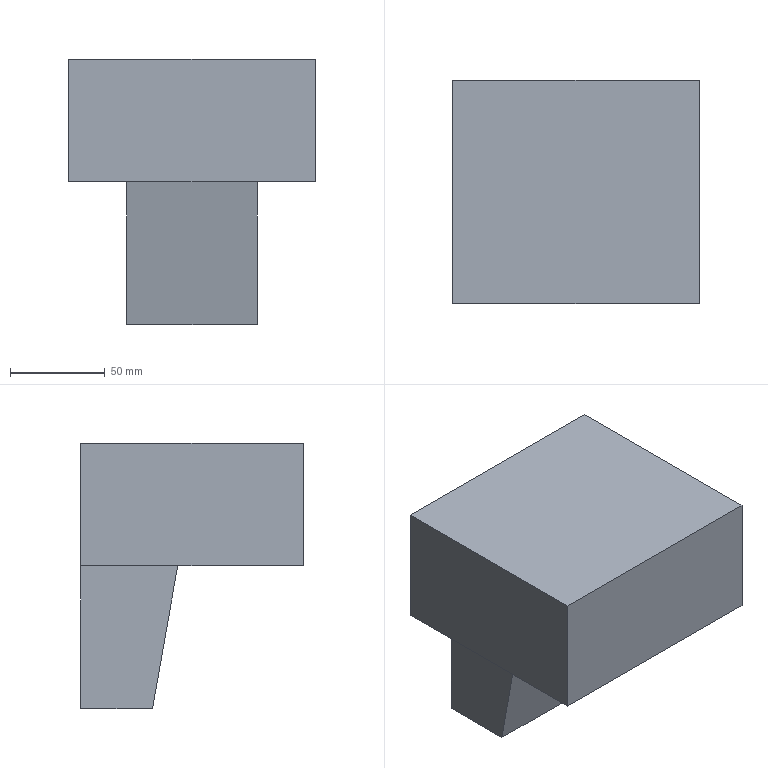Part | Creo | 1 solid | 10 faces | box 130 x 117.574 x 140 mm | volume 1218802 mm3 | plane 10
STEP:
#1=CARTESIAN_POINT('',(0.,0.,0.));
#2=DIRECTION('',(0.,0.,1.));
#3=DIRECTION('',(1.,0.,0.));
#4=AXIS2_PLACEMENT_3D('',#1,#2,#3);
#5=CARTESIAN_POINT('',(-59.275,152.799,-28.441));
#6=VERTEX_POINT('',#5);
#7=CARTESIAN_POINT('',(70.725,152.799,-28.441));
#8=VERTEX_POINT('',#7);
#9=CARTESIAN_POINT('',(-59.275,152.799,-28.441));
#10=DIRECTION('',(1.,0.000000015,0.));
#11=VECTOR('',#10,130.);
#12=LINE('',#9,#11);
#13=EDGE_CURVE('',#6,#8,#12,.T.);
#14=ORIENTED_EDGE('',*,*,#13,.T.);
#15=CARTESIAN_POINT('',(70.725,270.373,-28.441));
#16=VERTEX_POINT('',#15);
#17=CARTESIAN_POINT('',(70.725,270.373,-28.441));
#18=DIRECTION('',(0.,-1.,0.));
#19=VECTOR('',#18,117.574);
#20=LINE('',#17,#19);
#21=EDGE_CURVE('',#16,#8,#20,.T.);
#22=ORIENTED_EDGE('',*,*,#21,.F.);
#23=CARTESIAN_POINT('',(40.118,270.373,-28.441));
#24=VERTEX_POINT('',#23);
#25=CARTESIAN_POINT('',(70.725,270.373,-28.441));
#26=DIRECTION('',(-1.,0.,0.));
#27=VECTOR('',#26,30.607);
#28=LINE('',#25,#27);
#29=EDGE_CURVE('',#16,#24,#28,.T.);
#30=ORIENTED_EDGE('',*,*,#29,.T.);
#31=CARTESIAN_POINT('',(40.118,219.12,-28.441));
#32=VERTEX_POINT('',#31);
#33=CARTESIAN_POINT('',(40.118,219.12,-28.441));
#34=DIRECTION('',(0.,1.,0.));
#35=VECTOR('',#34,51.252);
#36=LINE('',#33,#35);
#37=EDGE_CURVE('',#32,#24,#36,.T.);
#38=ORIENTED_EDGE('',*,*,#37,.F.);
#39=CARTESIAN_POINT('',(-28.668,219.12,-28.441));
#40=VERTEX_POINT('',#39);
#41=CARTESIAN_POINT('',(-28.668,219.12,-28.441));
#42=DIRECTION('',(1.,0.,0.));
#43=VECTOR('',#42,68.786);
#44=LINE('',#41,#43);
#45=EDGE_CURVE('',#40,#32,#44,.T.);
#46=ORIENTED_EDGE('',*,*,#45,.F.);
#47=CARTESIAN_POINT('',(-28.668,270.373,-28.441));
#48=VERTEX_POINT('',#47);
#49=CARTESIAN_POINT('',(-28.668,270.373,-28.441));
#50=DIRECTION('',(0.,-1.,0.));
#51=VECTOR('',#50,51.252);
#52=LINE('',#49,#51);
#53=EDGE_CURVE('',#48,#40,#52,.T.);
#54=ORIENTED_EDGE('',*,*,#53,.F.);
#55=CARTESIAN_POINT('',(-59.275,270.373,-28.441));
#56=VERTEX_POINT('',#55);
#57=CARTESIAN_POINT('',(-28.668,270.373,-28.441));
#58=DIRECTION('',(-1.,0.,0.));
#59=VECTOR('',#58,30.607);
#60=LINE('',#57,#59);
#61=EDGE_CURVE('',#48,#56,#60,.T.);
#62=ORIENTED_EDGE('',*,*,#61,.T.);
#63=CARTESIAN_POINT('',(-59.275,270.373,-28.441));
#64=DIRECTION('',(0.,-1.,0.));
#65=VECTOR('',#64,117.574);
#66=LINE('',#63,#65);
#67=EDGE_CURVE('',#56,#6,#66,.T.);
#68=ORIENTED_EDGE('',*,*,#67,.T.);
#69=EDGE_LOOP('',(#14,#22,#30,#38,#46,#54,#62,#68));
#70=FACE_OUTER_BOUND('',#69,.F.);
#71=CARTESIAN_POINT('',(464.101,-434.627,-28.441));
#72=DIRECTION('',(0.,0.,-1.));
#73=DIRECTION('',(-1.,0.,0.));
#74=AXIS2_PLACEMENT_3D('',#71,#72,#73);
#75=PLANE('',#74);
#76=ADVANCED_FACE('',(#70),#75,.T.);
#77=CARTESIAN_POINT('',(-59.275,152.799,36.165));
#78=VERTEX_POINT('',#77);
#79=CARTESIAN_POINT('',(70.725,152.799,36.165));
#80=VERTEX_POINT('',#79);
#81=CARTESIAN_POINT('',(-59.275,152.799,36.165));
#82=DIRECTION('',(1.,0.000000015,0.));
#83=VECTOR('',#82,130.);
#84=LINE('',#81,#83);
#85=EDGE_CURVE('',#78,#80,#84,.T.);
#86=ORIENTED_EDGE('',*,*,#85,.T.);
#87=CARTESIAN_POINT('',(70.725,152.799,-28.441));
#88=DIRECTION('',(0.,0.,1.));
#89=VECTOR('',#88,64.606);
#90=LINE('',#87,#89);
#91=EDGE_CURVE('',#8,#80,#90,.T.);
#92=ORIENTED_EDGE('',*,*,#91,.F.);
#93=ORIENTED_EDGE('',*,*,#13,.F.);
#94=CARTESIAN_POINT('',(-59.275,152.799,-28.441));
#95=DIRECTION('',(0.,0.,1.));
#96=VECTOR('',#95,64.606);
#97=LINE('',#94,#96);
#98=EDGE_CURVE('',#6,#78,#97,.T.);
#99=ORIENTED_EDGE('',*,*,#98,.T.);
#100=EDGE_LOOP('',(#86,#92,#93,#99));
#101=FACE_OUTER_BOUND('',#100,.F.);
#102=CARTESIAN_POINT('',(57.885,152.799,12.059));
#103=DIRECTION('',(0.000000015,-1.,0.));
#104=DIRECTION('',(1.,0.000000015,0.));
#105=AXIS2_PLACEMENT_3D('',#102,#103,#104);
#106=PLANE('',#105);
#107=ADVANCED_FACE('',(#101),#106,.T.);
#108=CARTESIAN_POINT('',(-59.275,270.373,36.165));
#109=VERTEX_POINT('',#108);
#110=CARTESIAN_POINT('',(-59.275,270.373,36.165));
#111=DIRECTION('',(0.,-1.,0.));
#112=VECTOR('',#111,117.574);
#113=LINE('',#110,#112);
#114=EDGE_CURVE('',#109,#78,#113,.T.);
#115=ORIENTED_EDGE('',*,*,#114,.F.);
#116=CARTESIAN_POINT('',(70.725,270.373,36.165));
#117=VERTEX_POINT('',#116);
#118=CARTESIAN_POINT('',(70.725,270.373,36.165));
#119=DIRECTION('',(-1.,0.,0.));
#120=VECTOR('',#119,130.);
#121=LINE('',#118,#120);
#122=EDGE_CURVE('',#117,#109,#121,.T.);
#123=ORIENTED_EDGE('',*,*,#122,.F.);
#124=CARTESIAN_POINT('',(70.725,270.373,36.165));
#125=DIRECTION('',(0.,-1.,0.));
#126=VECTOR('',#125,117.574);
#127=LINE('',#124,#126);
#128=EDGE_CURVE('',#117,#80,#127,.T.);
#129=ORIENTED_EDGE('',*,*,#128,.T.);
#130=ORIENTED_EDGE('',*,*,#85,.F.);
#131=EDGE_LOOP('',(#115,#123,#129,#130));
#132=FACE_OUTER_BOUND('',#131,.F.);
#133=CARTESIAN_POINT('',(5.725,165.833,36.165));
#134=DIRECTION('',(0.,0.,1.));
#135=DIRECTION('',(1.,0.,0.));
#136=AXIS2_PLACEMENT_3D('',#133,#134,#135);
#137=PLANE('',#136);
#138=ADVANCED_FACE('',(#132),#137,.T.);
#139=ORIENTED_EDGE('',*,*,#67,.F.);
#140=CARTESIAN_POINT('',(-59.275,270.373,-28.441));
#141=DIRECTION('',(0.,0.,1.));
#142=VECTOR('',#141,64.606);
#143=LINE('',#140,#142);
#144=EDGE_CURVE('',#56,#109,#143,.T.);
#145=ORIENTED_EDGE('',*,*,#144,.T.);
#146=ORIENTED_EDGE('',*,*,#114,.T.);
#147=ORIENTED_EDGE('',*,*,#98,.F.);
#148=EDGE_LOOP('',(#139,#145,#146,#147));
#149=FACE_OUTER_BOUND('',#148,.F.);
#150=CARTESIAN_POINT('',(-59.275,270.373,36.165));
#151=DIRECTION('',(1.,0.,0.));
#152=DIRECTION('',(0.,0.,-1.));
#153=AXIS2_PLACEMENT_3D('',#150,#151,#152);
#154=PLANE('',#153);
#155=ADVANCED_FACE('',(#149),#154,.F.);
#156=CARTESIAN_POINT('',(40.118,270.373,-103.835));
#157=VERTEX_POINT('',#156);
#158=CARTESIAN_POINT('',(-28.668,270.373,-103.835));
#159=VERTEX_POINT('',#158);
#160=CARTESIAN_POINT('',(40.118,270.373,-103.835));
#161=DIRECTION('',(-1.,0.,0.));
#162=VECTOR('',#161,68.786);
#163=LINE('',#160,#162);
#164=EDGE_CURVE('',#157,#159,#163,.T.);
#165=ORIENTED_EDGE('',*,*,#164,.F.);
#166=CARTESIAN_POINT('',(40.118,270.373,-28.441));
#167=DIRECTION('',(0.,0.,-1.));
#168=VECTOR('',#167,75.394);
#169=LINE('',#166,#168);
#170=EDGE_CURVE('',#24,#157,#169,.T.);
#171=ORIENTED_EDGE('',*,*,#170,.F.);
#172=ORIENTED_EDGE('',*,*,#29,.F.);
#173=CARTESIAN_POINT('',(70.725,270.373,-28.441));
#174=DIRECTION('',(0.,0.,1.));
#175=VECTOR('',#174,64.606);
#176=LINE('',#173,#175);
#177=EDGE_CURVE('',#16,#117,#176,.T.);
#178=ORIENTED_EDGE('',*,*,#177,.T.);
#179=ORIENTED_EDGE('',*,*,#122,.T.);
#180=ORIENTED_EDGE('',*,*,#144,.F.);
#181=ORIENTED_EDGE('',*,*,#61,.F.);
#182=CARTESIAN_POINT('',(-28.668,270.373,-28.441));
#183=DIRECTION('',(0.,0.,-1.));
#184=VECTOR('',#183,75.394);
#185=LINE('',#182,#184);
#186=EDGE_CURVE('',#48,#159,#185,.T.);
#187=ORIENTED_EDGE('',*,*,#186,.T.);
#188=EDGE_LOOP('',(#165,#171,#172,#178,#179,#180,#181,#187));
#189=FACE_OUTER_BOUND('',#188,.F.);
#190=CARTESIAN_POINT('',(5.725,270.373,-138.014));
#191=DIRECTION('',(0.,1.,0.));
#192=DIRECTION('',(0.,0.,1.));
#193=AXIS2_PLACEMENT_3D('',#190,#191,#192);
#194=PLANE('',#193);
#195=ADVANCED_FACE('',(#189),#194,.T.);
#196=ORIENTED_EDGE('',*,*,#164,.T.);
#197=CARTESIAN_POINT('',(-28.668,232.414,-103.835));
#198=VERTEX_POINT('',#197);
#199=CARTESIAN_POINT('',(-28.668,270.373,-103.835));
#200=DIRECTION('',(0.,-1.,0.));
#201=VECTOR('',#200,37.958);
#202=LINE('',#199,#201);
#203=EDGE_CURVE('',#159,#198,#202,.T.);
#204=ORIENTED_EDGE('',*,*,#203,.T.);
#205=CARTESIAN_POINT('',(40.118,232.414,-103.835));
#206=VERTEX_POINT('',#205);
#207=CARTESIAN_POINT('',(40.118,232.414,-103.835));
#208=DIRECTION('',(-1.,0.,0.));
#209=VECTOR('',#208,68.786);
#210=LINE('',#207,#209);
#211=EDGE_CURVE('',#206,#198,#210,.T.);
#212=ORIENTED_EDGE('',*,*,#211,.F.);
#213=CARTESIAN_POINT('',(40.118,232.414,-103.835));
#214=DIRECTION('',(0.,1.,0.));
#215=VECTOR('',#214,37.958);
#216=LINE('',#213,#215);
#217=EDGE_CURVE('',#206,#157,#216,.T.);
#218=ORIENTED_EDGE('',*,*,#217,.T.);
#219=EDGE_LOOP('',(#196,#204,#212,#218));
#220=FACE_OUTER_BOUND('',#219,.F.);
#221=CARTESIAN_POINT('',(-59.275,270.373,-103.835));
#222=DIRECTION('',(0.,0.,1.));
#223=DIRECTION('',(1.,0.,0.));
#224=AXIS2_PLACEMENT_3D('',#221,#222,#223);
#225=PLANE('',#224);
#226=ADVANCED_FACE('',(#220),#225,.F.);
#227=ORIENTED_EDGE('',*,*,#203,.F.);
#228=ORIENTED_EDGE('',*,*,#186,.F.);
#229=ORIENTED_EDGE('',*,*,#53,.T.);
#230=CARTESIAN_POINT('',(-28.668,232.414,-103.835));
#231=DIRECTION('',(0.,-0.1736,0.9848));
#232=VECTOR('',#231,76.557);
#233=LINE('',#230,#232);
#234=EDGE_CURVE('',#198,#40,#233,.T.);
#235=ORIENTED_EDGE('',*,*,#234,.F.);
#236=EDGE_LOOP('',(#227,#228,#229,#235));
#237=FACE_OUTER_BOUND('',#236,.F.);
#238=CARTESIAN_POINT('',(-28.668,165.833,-138.014));
#239=DIRECTION('',(-1.,0.,0.));
#240=DIRECTION('',(0.,0.,1.));
#241=AXIS2_PLACEMENT_3D('',#238,#239,#240);
#242=PLANE('',#241);
#243=ADVANCED_FACE('',(#237),#242,.T.);
#244=ORIENTED_EDGE('',*,*,#234,.T.);
#245=ORIENTED_EDGE('',*,*,#45,.T.);
#246=CARTESIAN_POINT('',(40.118,219.12,-28.441));
#247=DIRECTION('',(0.,0.1736,-0.9848));
#248=VECTOR('',#247,76.557);
#249=LINE('',#246,#248);
#250=EDGE_CURVE('',#32,#206,#249,.T.);
#251=ORIENTED_EDGE('',*,*,#250,.T.);
#252=ORIENTED_EDGE('',*,*,#211,.T.);
#253=EDGE_LOOP('',(#244,#245,#251,#252));
#254=FACE_OUTER_BOUND('',#253,.F.);
#255=CARTESIAN_POINT('',(-335.899,236.585,-127.489));
#256=DIRECTION('',(0.,-0.9848,-0.1736));
#257=DIRECTION('',(0.,0.1736,-0.9848));
#258=AXIS2_PLACEMENT_3D('',#255,#256,#257);
#259=PLANE('',#258);
#260=ADVANCED_FACE('',(#254),#259,.T.);
#261=ORIENTED_EDGE('',*,*,#217,.F.);
#262=ORIENTED_EDGE('',*,*,#250,.F.);
#263=ORIENTED_EDGE('',*,*,#37,.T.);
#264=ORIENTED_EDGE('',*,*,#170,.T.);
#265=EDGE_LOOP('',(#261,#262,#263,#264));
#266=FACE_OUTER_BOUND('',#265,.F.);
#267=CARTESIAN_POINT('',(40.118,165.833,-138.014));
#268=DIRECTION('',(1.,0.,0.));
#269=DIRECTION('',(0.,0.,-1.));
#270=AXIS2_PLACEMENT_3D('',#267,#268,#269);
#271=PLANE('',#270);
#272=ADVANCED_FACE('',(#266),#271,.T.);
#273=ORIENTED_EDGE('',*,*,#91,.T.);
#274=ORIENTED_EDGE('',*,*,#128,.F.);
#275=ORIENTED_EDGE('',*,*,#177,.F.);
#276=ORIENTED_EDGE('',*,*,#21,.T.);
#277=EDGE_LOOP('',(#273,#274,#275,#276));
#278=FACE_OUTER_BOUND('',#277,.F.);
#279=CARTESIAN_POINT('',(70.725,270.373,36.165));
#280=DIRECTION('',(1.,0.,0.));
#281=DIRECTION('',(0.,0.,-1.));
#282=AXIS2_PLACEMENT_3D('',#279,#280,#281);
#283=PLANE('',#282);
#284=ADVANCED_FACE('',(#278),#283,.T.);
#285=CLOSED_SHELL('',(#76,#107,#138,#155,#195,#226,#243,#260,#272,#284));
#286=MANIFOLD_SOLID_BREP('',#285);
#287=(LENGTH_UNIT()NAMED_UNIT(*)SI_UNIT(.MILLI.,.METRE.));
#288=UNCERTAINTY_MEASURE_WITH_UNIT(LENGTH_MEASURE(0.02243),#287,'','');
#289=(NAMED_UNIT(*)PLANE_ANGLE_UNIT()SI_UNIT($,.RADIAN.));
#290=PLANE_ANGLE_MEASURE_WITH_UNIT(PLANE_ANGLE_MEASURE(0.01745),#289);
#291=(CONVERSION_BASED_UNIT('DEGREE',#290)NAMED_UNIT(*)PLANE_ANGLE_UNIT());
#292=(NAMED_UNIT(*)SI_UNIT($,.STERADIAN.)SOLID_ANGLE_UNIT());
#293=(GEOMETRIC_REPRESENTATION_CONTEXT(3)GLOBAL_UNCERTAINTY_ASSIGNED_CONTEXT((#288))GLOBAL_UNIT_ASSIGNED_CONTEXT((#287,#291,#292))REPRESENTATION_CONTEXT('',''));
#294=ADVANCED_BREP_SHAPE_REPRESENTATION('',(#4,#286),#293);